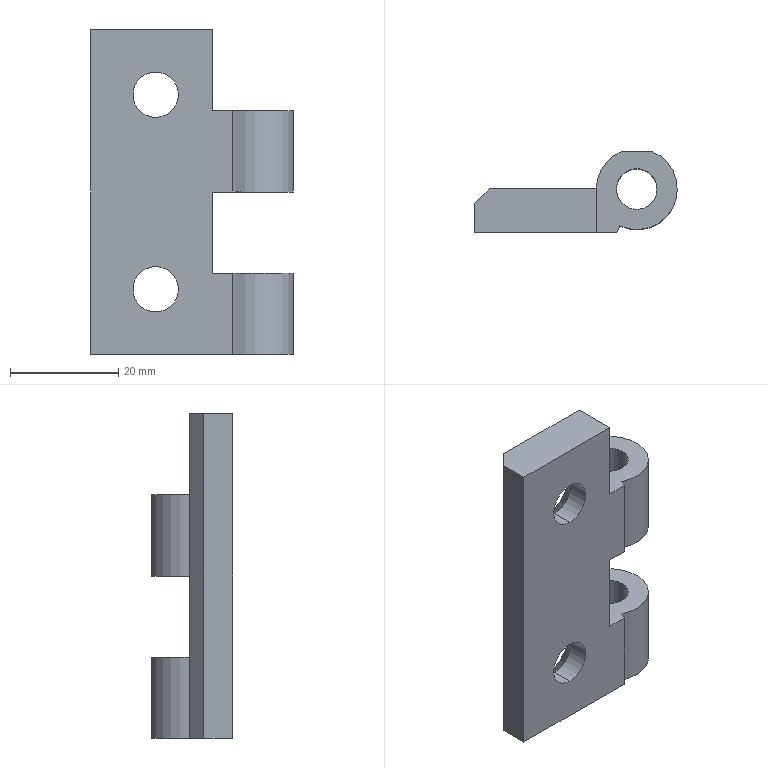Part | SolidWorks | features BaseBody 1 | 1 solid | 31 faces | box 37.5 x 15 x 60 mm | volume 13445 mm3 | plane 15 | cylinder 12 | cone 4 | commonest cylinder face diameters 7.5 x4 8.4 x4 15 x4
STEP:
#1=CARTESIAN_POINT('',(-18.,-4.05,-7.8));
#2=VERTEX_POINT('',#1);
#3=CARTESIAN_POINT('',(-18.,-4.05,-16.2));
#4=VERTEX_POINT('',#3);
#5=CARTESIAN_POINT('',(-18.,-4.05,-12.));
#6=DIRECTION('',(0.,-1.,0.));
#7=DIRECTION('',(0.,0.,-1.));
#8=AXIS2_PLACEMENT_3D('',#5,#6,#7);
#9=CIRCLE('',#8,4.2);
#10=EDGE_CURVE('',#2,#4,#9,.T.);
#11=ORIENTED_EDGE('',*,*,#10,.F.);
#12=CARTESIAN_POINT('',(-18.,-8.,-7.8));
#13=VERTEX_POINT('',#12);
#14=CARTESIAN_POINT('',(-18.,50.,-7.8));
#15=DIRECTION('',(0.,-1.,0.));
#16=VECTOR('',#15,1000.);
#17=LINE('',#14,#16);
#18=EDGE_CURVE('',#2,#13,#17,.T.);
#19=ORIENTED_EDGE('',*,*,#18,.T.);
#20=CARTESIAN_POINT('',(-18.,-8.,-16.2));
#21=VERTEX_POINT('',#20);
#22=CARTESIAN_POINT('',(-18.,-8.,-12.));
#23=DIRECTION('',(0.,-1.,0.));
#24=DIRECTION('',(0.,0.,-1.));
#25=AXIS2_PLACEMENT_3D('',#22,#23,#24);
#26=CIRCLE('',#25,4.2);
#27=EDGE_CURVE('',#13,#21,#26,.T.);
#28=ORIENTED_EDGE('',*,*,#27,.T.);
#29=CARTESIAN_POINT('',(-18.,50.,-16.2));
#30=DIRECTION('',(0.,-1.,0.));
#31=VECTOR('',#30,1000.);
#32=LINE('',#29,#31);
#33=EDGE_CURVE('',#4,#21,#32,.T.);
#34=ORIENTED_EDGE('',*,*,#33,.F.);
#35=EDGE_LOOP('',(#11,#19,#28,#34));
#36=FACE_OUTER_BOUND('',#35,.T.);
#37=CARTESIAN_POINT('',(-18.,50.,-12.));
#38=DIRECTION('',(0.,-1.,0.));
#39=DIRECTION('',(0.,0.,-1.));
#40=AXIS2_PLACEMENT_3D('',#37,#38,#39);
#41=CYLINDRICAL_SURFACE('',#40,4.2);
#42=ADVANCED_FACE('',(#36),#41,.F.);
#43=CARTESIAN_POINT('',(-18.,-4.05,-43.8));
#44=VERTEX_POINT('',#43);
#45=CARTESIAN_POINT('',(-18.,-4.05,-52.2));
#46=VERTEX_POINT('',#45);
#47=CARTESIAN_POINT('',(-18.,-4.05,-48.));
#48=DIRECTION('',(0.,-1.,0.));
#49=DIRECTION('',(0.,0.,-1.));
#50=AXIS2_PLACEMENT_3D('',#47,#48,#49);
#51=CIRCLE('',#50,4.2);
#52=EDGE_CURVE('',#44,#46,#51,.T.);
#53=ORIENTED_EDGE('',*,*,#52,.F.);
#54=CARTESIAN_POINT('',(-18.,-8.,-43.8));
#55=VERTEX_POINT('',#54);
#56=CARTESIAN_POINT('',(-18.,50.,-43.8));
#57=DIRECTION('',(0.,-1.,0.));
#58=VECTOR('',#57,1000.);
#59=LINE('',#56,#58);
#60=EDGE_CURVE('',#44,#55,#59,.T.);
#61=ORIENTED_EDGE('',*,*,#60,.T.);
#62=CARTESIAN_POINT('',(-18.,-8.,-52.2));
#63=VERTEX_POINT('',#62);
#64=CARTESIAN_POINT('',(-18.,-8.,-48.));
#65=DIRECTION('',(0.,-1.,0.));
#66=DIRECTION('',(0.,0.,-1.));
#67=AXIS2_PLACEMENT_3D('',#64,#65,#66);
#68=CIRCLE('',#67,4.2);
#69=EDGE_CURVE('',#55,#63,#68,.T.);
#70=ORIENTED_EDGE('',*,*,#69,.T.);
#71=CARTESIAN_POINT('',(-18.,50.,-52.2));
#72=DIRECTION('',(0.,-1.,0.));
#73=VECTOR('',#72,1000.);
#74=LINE('',#71,#73);
#75=EDGE_CURVE('',#46,#63,#74,.T.);
#76=ORIENTED_EDGE('',*,*,#75,.F.);
#77=EDGE_LOOP('',(#53,#61,#70,#76));
#78=FACE_OUTER_BOUND('',#77,.T.);
#79=CARTESIAN_POINT('',(-18.,50.,-48.));
#80=DIRECTION('',(0.,-1.,0.));
#81=DIRECTION('',(0.,0.,-1.));
#82=AXIS2_PLACEMENT_3D('',#79,#80,#81);
#83=CYLINDRICAL_SURFACE('',#82,4.2);
#84=ADVANCED_FACE('',(#78),#83,.F.);
#85=ORIENTED_EDGE('',*,*,#10,.T.);
#86=CARTESIAN_POINT('',(-18.,0.,-20.25));
#87=VERTEX_POINT('',#86);
#88=CARTESIAN_POINT('',(-18.,0.,-20.25));
#89=DIRECTION('',(0.,0.7071,-0.7071));
#90=VECTOR('',#89,1000.);
#91=LINE('',#88,#90);
#92=EDGE_CURVE('',#4,#87,#91,.T.);
#93=ORIENTED_EDGE('',*,*,#92,.T.);
#94=CARTESIAN_POINT('',(-18.,0.,-3.75));
#95=VERTEX_POINT('',#94);
#96=CARTESIAN_POINT('',(-18.,0.,-12.));
#97=DIRECTION('',(0.,-1.,0.));
#98=DIRECTION('',(0.,0.,1.));
#99=AXIS2_PLACEMENT_3D('',#96,#97,#98);
#100=CIRCLE('',#99,8.25);
#101=EDGE_CURVE('',#95,#87,#100,.T.);
#102=ORIENTED_EDGE('',*,*,#101,.F.);
#103=CARTESIAN_POINT('',(-18.,0.,-3.75));
#104=DIRECTION('',(0.,0.7071,0.7071));
#105=VECTOR('',#104,1000.);
#106=LINE('',#103,#105);
#107=EDGE_CURVE('',#2,#95,#106,.T.);
#108=ORIENTED_EDGE('',*,*,#107,.F.);
#109=EDGE_LOOP('',(#85,#93,#102,#108));
#110=FACE_OUTER_BOUND('',#109,.T.);
#111=CARTESIAN_POINT('',(-18.,0.,-12.));
#112=DIRECTION('',(0.,1.,0.));
#113=DIRECTION('',(0.,0.,1.));
#114=AXIS2_PLACEMENT_3D('',#111,#112,#113);
#115=CONICAL_SURFACE('',#114,8.25,0.7854);
#116=ADVANCED_FACE('',(#110),#115,.F.);
#117=ORIENTED_EDGE('',*,*,#52,.T.);
#118=CARTESIAN_POINT('',(-18.,0.,-56.25));
#119=VERTEX_POINT('',#118);
#120=CARTESIAN_POINT('',(-18.,0.,-56.25));
#121=DIRECTION('',(0.,0.7071,-0.7071));
#122=VECTOR('',#121,1000.);
#123=LINE('',#120,#122);
#124=EDGE_CURVE('',#46,#119,#123,.T.);
#125=ORIENTED_EDGE('',*,*,#124,.T.);
#126=CARTESIAN_POINT('',(-18.,0.,-39.75));
#127=VERTEX_POINT('',#126);
#128=CARTESIAN_POINT('',(-18.,0.,-48.));
#129=DIRECTION('',(0.,-1.,0.));
#130=DIRECTION('',(0.,0.,1.));
#131=AXIS2_PLACEMENT_3D('',#128,#129,#130);
#132=CIRCLE('',#131,8.25);
#133=EDGE_CURVE('',#127,#119,#132,.T.);
#134=ORIENTED_EDGE('',*,*,#133,.F.);
#135=CARTESIAN_POINT('',(-18.,0.,-39.75));
#136=DIRECTION('',(0.,0.7071,0.7071));
#137=VECTOR('',#136,1000.);
#138=LINE('',#135,#137);
#139=EDGE_CURVE('',#44,#127,#138,.T.);
#140=ORIENTED_EDGE('',*,*,#139,.F.);
#141=EDGE_LOOP('',(#117,#125,#134,#140));
#142=FACE_OUTER_BOUND('',#141,.T.);
#143=CARTESIAN_POINT('',(-18.,0.,-48.));
#144=DIRECTION('',(0.,1.,0.));
#145=DIRECTION('',(0.,0.,1.));
#146=AXIS2_PLACEMENT_3D('',#143,#144,#145);
#147=CONICAL_SURFACE('',#146,8.25,0.7854);
#148=ADVANCED_FACE('',(#142),#147,.F.);
#149=CARTESIAN_POINT('',(3.75,0.,-45.));
#150=VERTEX_POINT('',#149);
#151=CARTESIAN_POINT('',(-3.75,0.,-45.));
#152=VERTEX_POINT('',#151);
#153=CARTESIAN_POINT('',(0.,0.,-45.));
#154=DIRECTION('',(0.,0.,-1.));
#155=DIRECTION('',(-1.,0.,0.));
#156=AXIS2_PLACEMENT_3D('',#153,#154,#155);
#157=CIRCLE('',#156,3.75);
#158=EDGE_CURVE('',#150,#152,#157,.T.);
#159=ORIENTED_EDGE('',*,*,#158,.F.);
#160=CARTESIAN_POINT('',(3.75,0.,-60.));
#161=VERTEX_POINT('',#160);
#162=CARTESIAN_POINT('',(3.75,0.,-60.));
#163=DIRECTION('',(0.,0.,-1.));
#164=VECTOR('',#163,1000.);
#165=LINE('',#162,#164);
#166=EDGE_CURVE('',#150,#161,#165,.T.);
#167=ORIENTED_EDGE('',*,*,#166,.T.);
#168=CARTESIAN_POINT('',(-3.75,0.,-60.));
#169=VERTEX_POINT('',#168);
#170=CARTESIAN_POINT('',(0.,0.,-60.));
#171=DIRECTION('',(0.,0.,1.));
#172=DIRECTION('',(-1.,0.,0.));
#173=AXIS2_PLACEMENT_3D('',#170,#171,#172);
#174=CIRCLE('',#173,3.75);
#175=EDGE_CURVE('',#169,#161,#174,.T.);
#176=ORIENTED_EDGE('',*,*,#175,.F.);
#177=CARTESIAN_POINT('',(-3.75,0.,-60.));
#178=DIRECTION('',(0.,0.,-1.));
#179=VECTOR('',#178,1000.);
#180=LINE('',#177,#179);
#181=EDGE_CURVE('',#152,#169,#180,.T.);
#182=ORIENTED_EDGE('',*,*,#181,.F.);
#183=EDGE_LOOP('',(#159,#167,#176,#182));
#184=FACE_OUTER_BOUND('',#183,.T.);
#185=CARTESIAN_POINT('',(0.,0.,-60.));
#186=DIRECTION('',(0.,0.,-1.));
#187=DIRECTION('',(-1.,0.,0.));
#188=AXIS2_PLACEMENT_3D('',#185,#186,#187);
#189=CYLINDRICAL_SURFACE('',#188,3.75);
#190=ADVANCED_FACE('',(#184),#189,.F.);
#191=CARTESIAN_POINT('',(3.75,0.,-15.));
#192=VERTEX_POINT('',#191);
#193=CARTESIAN_POINT('',(-3.75,0.,-15.));
#194=VERTEX_POINT('',#193);
#195=CARTESIAN_POINT('',(0.,0.,-15.));
#196=DIRECTION('',(0.,0.,-1.));
#197=DIRECTION('',(-1.,0.,0.));
#198=AXIS2_PLACEMENT_3D('',#195,#196,#197);
#199=CIRCLE('',#198,3.75);
#200=EDGE_CURVE('',#192,#194,#199,.T.);
#201=ORIENTED_EDGE('',*,*,#200,.F.);
#202=CARTESIAN_POINT('',(3.75,0.,-30.));
#203=VERTEX_POINT('',#202);
#204=CARTESIAN_POINT('',(3.75,0.,-60.));
#205=DIRECTION('',(0.,0.,-1.));
#206=VECTOR('',#205,1000.);
#207=LINE('',#204,#206);
#208=EDGE_CURVE('',#192,#203,#207,.T.);
#209=ORIENTED_EDGE('',*,*,#208,.T.);
#210=CARTESIAN_POINT('',(-3.75,0.,-30.));
#211=VERTEX_POINT('',#210);
#212=CARTESIAN_POINT('',(0.,0.,-30.));
#213=DIRECTION('',(0.,0.,1.));
#214=DIRECTION('',(-1.,0.,0.));
#215=AXIS2_PLACEMENT_3D('',#212,#213,#214);
#216=CIRCLE('',#215,3.75);
#217=EDGE_CURVE('',#211,#203,#216,.T.);
#218=ORIENTED_EDGE('',*,*,#217,.F.);
#219=CARTESIAN_POINT('',(-3.75,0.,-60.));
#220=DIRECTION('',(0.,0.,-1.));
#221=VECTOR('',#220,1000.);
#222=LINE('',#219,#221);
#223=EDGE_CURVE('',#194,#211,#222,.T.);
#224=ORIENTED_EDGE('',*,*,#223,.F.);
#225=EDGE_LOOP('',(#201,#209,#218,#224));
#226=FACE_OUTER_BOUND('',#225,.T.);
#227=CARTESIAN_POINT('',(0.,0.,-60.));
#228=DIRECTION('',(0.,0.,-1.));
#229=DIRECTION('',(-1.,0.,0.));
#230=AXIS2_PLACEMENT_3D('',#227,#228,#229);
#231=CYLINDRICAL_SURFACE('',#230,3.75);
#232=ADVANCED_FACE('',(#226),#231,.F.);
#233=CARTESIAN_POINT('',(-18.,-8.,-12.));
#234=DIRECTION('',(0.,-1.,0.));
#235=DIRECTION('',(0.,0.,-1.));
#236=AXIS2_PLACEMENT_3D('',#233,#234,#235);
#237=CIRCLE('',#236,4.2);
#238=EDGE_CURVE('',#21,#13,#237,.T.);
#239=ORIENTED_EDGE('',*,*,#238,.F.);
#240=ORIENTED_EDGE('',*,*,#27,.F.);
#241=EDGE_LOOP('',(#239,#240));
#242=FACE_BOUND('',#241,.T.);
#243=CARTESIAN_POINT('',(-18.,-8.,-48.));
#244=DIRECTION('',(0.,-1.,0.));
#245=DIRECTION('',(0.,0.,-1.));
#246=AXIS2_PLACEMENT_3D('',#243,#244,#245);
#247=CIRCLE('',#246,4.2);
#248=EDGE_CURVE('',#63,#55,#247,.T.);
#249=ORIENTED_EDGE('',*,*,#248,.F.);
#250=ORIENTED_EDGE('',*,*,#69,.F.);
#251=EDGE_LOOP('',(#249,#250));
#252=FACE_BOUND('',#251,.T.);
#253=CARTESIAN_POINT('',(-7.5,-8.,-30.));
#254=VERTEX_POINT('',#253);
#255=CARTESIAN_POINT('',(-7.5,-8.,-45.));
#256=VERTEX_POINT('',#255);
#257=CARTESIAN_POINT('',(-7.5,-8.,-60.));
#258=DIRECTION('',(0.,0.,-1.));
#259=VECTOR('',#258,1000.);
#260=LINE('',#257,#259);
#261=EDGE_CURVE('',#254,#256,#260,.T.);
#262=ORIENTED_EDGE('',*,*,#261,.F.);
#263=CARTESIAN_POINT('',(-3.75,-8.,-30.));
#264=VERTEX_POINT('',#263);
#265=CARTESIAN_POINT('',(-3.75,-8.,-30.));
#266=DIRECTION('',(-1.,0.,0.));
#267=VECTOR('',#266,1000.);
#268=LINE('',#265,#267);
#269=EDGE_CURVE('',#264,#254,#268,.T.);
#270=ORIENTED_EDGE('',*,*,#269,.F.);
#271=CARTESIAN_POINT('',(-3.75,-8.,-15.));
#272=VERTEX_POINT('',#271);
#273=CARTESIAN_POINT('',(-3.75,-8.,-60.));
#274=DIRECTION('',(0.,0.,-1.));
#275=VECTOR('',#274,1000.);
#276=LINE('',#273,#275);
#277=EDGE_CURVE('',#272,#264,#276,.T.);
#278=ORIENTED_EDGE('',*,*,#277,.F.);
#279=CARTESIAN_POINT('',(-7.5,-8.,-15.));
#280=VERTEX_POINT('',#279);
#281=CARTESIAN_POINT('',(-3.75,-8.,-15.));
#282=DIRECTION('',(1.,0.,0.));
#283=VECTOR('',#282,1000.);
#284=LINE('',#281,#283);
#285=EDGE_CURVE('',#280,#272,#284,.T.);
#286=ORIENTED_EDGE('',*,*,#285,.F.);
#287=CARTESIAN_POINT('',(-7.5,-8.,0.));
#288=VERTEX_POINT('',#287);
#289=CARTESIAN_POINT('',(-7.5,-8.,-60.));
#290=DIRECTION('',(0.,0.,-1.));
#291=VECTOR('',#290,1000.);
#292=LINE('',#289,#291);
#293=EDGE_CURVE('',#288,#280,#292,.T.);
#294=ORIENTED_EDGE('',*,*,#293,.F.);
#295=CARTESIAN_POINT('',(-30.,-8.,0.));
#296=VERTEX_POINT('',#295);
#297=CARTESIAN_POINT('',(-3.75,-8.,0.));
#298=DIRECTION('',(1.,0.,0.));
#299=VECTOR('',#298,1000.);
#300=LINE('',#297,#299);
#301=EDGE_CURVE('',#296,#288,#300,.T.);
#302=ORIENTED_EDGE('',*,*,#301,.F.);
#303=CARTESIAN_POINT('',(-30.,-8.,-60.));
#304=VERTEX_POINT('',#303);
#305=CARTESIAN_POINT('',(-30.,-8.,-60.));
#306=DIRECTION('',(0.,0.,1.));
#307=VECTOR('',#306,1000.);
#308=LINE('',#305,#307);
#309=EDGE_CURVE('',#304,#296,#308,.T.);
#310=ORIENTED_EDGE('',*,*,#309,.F.);
#311=CARTESIAN_POINT('',(-3.75,-8.,-60.));
#312=VERTEX_POINT('',#311);
#313=CARTESIAN_POINT('',(-3.75,-8.,-60.));
#314=DIRECTION('',(-1.,0.,0.));
#315=VECTOR('',#314,1000.);
#316=LINE('',#313,#315);
#317=EDGE_CURVE('',#312,#304,#316,.T.);
#318=ORIENTED_EDGE('',*,*,#317,.F.);
#319=CARTESIAN_POINT('',(-3.75,-8.,-45.));
#320=VERTEX_POINT('',#319);
#321=CARTESIAN_POINT('',(-3.75,-8.,-60.));
#322=DIRECTION('',(0.,0.,-1.));
#323=VECTOR('',#322,1000.);
#324=LINE('',#321,#323);
#325=EDGE_CURVE('',#320,#312,#324,.T.);
#326=ORIENTED_EDGE('',*,*,#325,.F.);
#327=CARTESIAN_POINT('',(-3.75,-8.,-45.));
#328=DIRECTION('',(1.,0.,0.));
#329=VECTOR('',#328,1000.);
#330=LINE('',#327,#329);
#331=EDGE_CURVE('',#256,#320,#330,.T.);
#332=ORIENTED_EDGE('',*,*,#331,.F.);
#333=EDGE_LOOP('',(#262,#270,#278,#286,#294,#302,#310,#318,#326,#332));
#334=FACE_OUTER_BOUND('',#333,.T.);
#335=CARTESIAN_POINT('',(-3.75,-8.,-60.));
#336=DIRECTION('',(0.,1.,0.));
#337=DIRECTION('',(0.,0.,1.));
#338=AXIS2_PLACEMENT_3D('',#335,#336,#337);
#339=PLANE('',#338);
#340=ADVANCED_FACE('',(#242,#252,#334),#339,.F.);
#341=ORIENTED_EDGE('',*,*,#18,.F.);
#342=CARTESIAN_POINT('',(-18.,-4.05,-12.));
#343=DIRECTION('',(0.,-1.,0.));
#344=DIRECTION('',(0.,0.,-1.));
#345=AXIS2_PLACEMENT_3D('',#342,#343,#344);
#346=CIRCLE('',#345,4.2);
#347=EDGE_CURVE('',#4,#2,#346,.T.);
#348=ORIENTED_EDGE('',*,*,#347,.F.);
#349=ORIENTED_EDGE('',*,*,#33,.T.);
#350=ORIENTED_EDGE('',*,*,#238,.T.);
#351=EDGE_LOOP('',(#341,#348,#349,#350));
#352=FACE_OUTER_BOUND('',#351,.T.);
#353=CARTESIAN_POINT('',(-18.,50.,-12.));
#354=DIRECTION('',(0.,-1.,0.));
#355=DIRECTION('',(0.,0.,-1.));
#356=AXIS2_PLACEMENT_3D('',#353,#354,#355);
#357=CYLINDRICAL_SURFACE('',#356,4.2);
#358=ADVANCED_FACE('',(#352),#357,.F.);
#359=ORIENTED_EDGE('',*,*,#60,.F.);
#360=CARTESIAN_POINT('',(-18.,-4.05,-48.));
#361=DIRECTION('',(0.,-1.,0.));
#362=DIRECTION('',(0.,0.,-1.));
#363=AXIS2_PLACEMENT_3D('',#360,#361,#362);
#364=CIRCLE('',#363,4.2);
#365=EDGE_CURVE('',#46,#44,#364,.T.);
#366=ORIENTED_EDGE('',*,*,#365,.F.);
#367=ORIENTED_EDGE('',*,*,#75,.T.);
#368=ORIENTED_EDGE('',*,*,#248,.T.);
#369=EDGE_LOOP('',(#359,#366,#367,#368));
#370=FACE_OUTER_BOUND('',#369,.T.);
#371=CARTESIAN_POINT('',(-18.,50.,-48.));
#372=DIRECTION('',(0.,-1.,0.));
#373=DIRECTION('',(0.,0.,-1.));
#374=AXIS2_PLACEMENT_3D('',#371,#372,#373);
#375=CYLINDRICAL_SURFACE('',#374,4.2);
#376=ADVANCED_FACE('',(#370),#375,.F.);
#377=CARTESIAN_POINT('',(0.,0.,-45.));
#378=DIRECTION('',(0.,0.,-1.));
#379=DIRECTION('',(-1.,0.,0.));
#380=AXIS2_PLACEMENT_3D('',#377,#378,#379);
#381=CIRCLE('',#380,3.75);
#382=EDGE_CURVE('',#152,#150,#381,.T.);
#383=ORIENTED_EDGE('',*,*,#382,.T.);
#384=ORIENTED_EDGE('',*,*,#158,.T.);
#385=EDGE_LOOP('',(#383,#384));
#386=FACE_BOUND('',#385,.T.);
#387=CARTESIAN_POINT('',(-2.693,7.,-45.));
#388=VERTEX_POINT('',#387);
#389=CARTESIAN_POINT('',(-7.5,0.,-45.));
#390=VERTEX_POINT('',#389);
#391=CARTESIAN_POINT('',(0.,0.,-45.));
#392=DIRECTION('',(0.,0.,1.));
#393=DIRECTION('',(-1.,0.,0.));
#394=AXIS2_PLACEMENT_3D('',#391,#392,#393);
#395=CIRCLE('',#394,7.5);
#396=EDGE_CURVE('',#388,#390,#395,.T.);
#397=ORIENTED_EDGE('',*,*,#396,.T.);
#398=CARTESIAN_POINT('',(-7.5,15.,-45.));
#399=DIRECTION('',(0.,-1.,0.));
#400=VECTOR('',#399,1000.);
#401=LINE('',#398,#400);
#402=EDGE_CURVE('',#390,#256,#401,.T.);
#403=ORIENTED_EDGE('',*,*,#402,.T.);
#404=ORIENTED_EDGE('',*,*,#331,.T.);
#405=CARTESIAN_POINT('',(-3.148,-6.808,-45.));
#406=VERTEX_POINT('',#405);
#407=CARTESIAN_POINT('',(-3.75,-8.,-45.));
#408=DIRECTION('',(0.451,0.8925,0.));
#409=VECTOR('',#408,1000.);
#410=LINE('',#407,#409);
#411=EDGE_CURVE('',#320,#406,#410,.T.);
#412=ORIENTED_EDGE('',*,*,#411,.T.);
#413=CARTESIAN_POINT('',(2.693,7.,-45.));
#414=VERTEX_POINT('',#413);
#415=CARTESIAN_POINT('',(0.,0.,-45.));
#416=DIRECTION('',(0.,0.,1.));
#417=DIRECTION('',(-1.,0.,0.));
#418=AXIS2_PLACEMENT_3D('',#415,#416,#417);
#419=CIRCLE('',#418,7.5);
#420=EDGE_CURVE('',#406,#414,#419,.T.);
#421=ORIENTED_EDGE('',*,*,#420,.T.);
#422=CARTESIAN_POINT('',(7.5,7.,-45.));
#423=DIRECTION('',(-1.,0.,0.));
#424=VECTOR('',#423,1000.);
#425=LINE('',#422,#424);
#426=EDGE_CURVE('',#414,#388,#425,.T.);
#427=ORIENTED_EDGE('',*,*,#426,.T.);
#428=EDGE_LOOP('',(#397,#403,#404,#412,#421,#427));
#429=FACE_OUTER_BOUND('',#428,.T.);
#430=CARTESIAN_POINT('',(7.5,15.,-45.));
#431=DIRECTION('',(0.,0.,1.));
#432=DIRECTION('',(1.,0.,0.));
#433=AXIS2_PLACEMENT_3D('',#430,#431,#432);
#434=PLANE('',#433);
#435=ADVANCED_FACE('',(#386,#429),#434,.T.);
#436=CARTESIAN_POINT('',(-7.5,0.,-30.));
#437=VERTEX_POINT('',#436);
#438=CARTESIAN_POINT('',(-7.5,0.,-45.));
#439=DIRECTION('',(0.,0.,1.));
#440=VECTOR('',#439,1000.);
#441=LINE('',#438,#440);
#442=EDGE_CURVE('',#390,#437,#441,.T.);
#443=ORIENTED_EDGE('',*,*,#442,.T.);
#444=CARTESIAN_POINT('',(-7.5,15.,-30.));
#445=DIRECTION('',(0.,-1.,0.));
#446=VECTOR('',#445,1000.);
#447=LINE('',#444,#446);
#448=EDGE_CURVE('',#437,#254,#447,.T.);
#449=ORIENTED_EDGE('',*,*,#448,.T.);
#450=ORIENTED_EDGE('',*,*,#261,.T.);
#451=ORIENTED_EDGE('',*,*,#402,.F.);
#452=EDGE_LOOP('',(#443,#449,#450,#451));
#453=FACE_OUTER_BOUND('',#452,.T.);
#454=CARTESIAN_POINT('',(-7.5,15.,-45.));
#455=DIRECTION('',(1.,0.,0.));
#456=DIRECTION('',(0.,0.,-1.));
#457=AXIS2_PLACEMENT_3D('',#454,#455,#456);
#458=PLANE('',#457);
#459=ADVANCED_FACE('',(#453),#458,.T.);
#460=ORIENTED_EDGE('',*,*,#217,.T.);
#461=CARTESIAN_POINT('',(0.,0.,-30.));
#462=DIRECTION('',(0.,0.,1.));
#463=DIRECTION('',(-1.,0.,0.));
#464=AXIS2_PLACEMENT_3D('',#461,#462,#463);
#465=CIRCLE('',#464,3.75);
#466=EDGE_CURVE('',#203,#211,#465,.T.);
#467=ORIENTED_EDGE('',*,*,#466,.T.);
#468=EDGE_LOOP('',(#460,#467));
#469=FACE_BOUND('',#468,.T.);
#470=CARTESIAN_POINT('',(2.693,7.,-30.));
#471=VERTEX_POINT('',#470);
#472=CARTESIAN_POINT('',(-3.148,-6.808,-30.));
#473=VERTEX_POINT('',#472);
#474=CARTESIAN_POINT('',(0.,0.,-30.));
#475=DIRECTION('',(0.,0.,-1.));
#476=DIRECTION('',(-1.,0.,0.));
#477=AXIS2_PLACEMENT_3D('',#474,#475,#476);
#478=CIRCLE('',#477,7.5);
#479=EDGE_CURVE('',#471,#473,#478,.T.);
#480=ORIENTED_EDGE('',*,*,#479,.T.);
#481=CARTESIAN_POINT('',(-3.148,-6.808,-30.));
#482=DIRECTION('',(-0.451,-0.8925,0.));
#483=VECTOR('',#482,1000.);
#484=LINE('',#481,#483);
#485=EDGE_CURVE('',#473,#264,#484,.T.);
#486=ORIENTED_EDGE('',*,*,#485,.T.);
#487=ORIENTED_EDGE('',*,*,#269,.T.);
#488=ORIENTED_EDGE('',*,*,#448,.F.);
#489=CARTESIAN_POINT('',(-2.693,7.,-30.));
#490=VERTEX_POINT('',#489);
#491=CARTESIAN_POINT('',(0.,0.,-30.));
#492=DIRECTION('',(0.,0.,-1.));
#493=DIRECTION('',(-1.,0.,0.));
#494=AXIS2_PLACEMENT_3D('',#491,#492,#493);
#495=CIRCLE('',#494,7.5);
#496=EDGE_CURVE('',#437,#490,#495,.T.);
#497=ORIENTED_EDGE('',*,*,#496,.T.);
#498=CARTESIAN_POINT('',(-7.5,7.,-30.));
#499=DIRECTION('',(1.,0.,0.));
#500=VECTOR('',#499,1000.);
#501=LINE('',#498,#500);
#502=EDGE_CURVE('',#490,#471,#501,.T.);
#503=ORIENTED_EDGE('',*,*,#502,.T.);
#504=EDGE_LOOP('',(#480,#486,#487,#488,#497,#503));
#505=FACE_OUTER_BOUND('',#504,.T.);
#506=CARTESIAN_POINT('',(-7.5,15.,-30.));
#507=DIRECTION('',(0.,0.,-1.));
#508=DIRECTION('',(-1.,0.,0.));
#509=AXIS2_PLACEMENT_3D('',#506,#507,#508);
#510=PLANE('',#509);
#511=ADVANCED_FACE('',(#469,#505),#510,.T.);
#512=CARTESIAN_POINT('',(-3.148,-6.808,-15.));
#513=VERTEX_POINT('',#512);
#514=CARTESIAN_POINT('',(-3.148,-6.808,-60.));
#515=DIRECTION('',(0.,0.,-1.));
#516=VECTOR('',#515,1000.);
#517=LINE('',#514,#516);
#518=EDGE_CURVE('',#513,#473,#517,.T.);
#519=ORIENTED_EDGE('',*,*,#518,.F.);
#520=CARTESIAN_POINT('',(-3.148,-6.808,-15.));
#521=DIRECTION('',(0.451,0.8925,0.));
#522=VECTOR('',#521,1000.);
#523=LINE('',#520,#522);
#524=EDGE_CURVE('',#272,#513,#523,.T.);
#525=ORIENTED_EDGE('',*,*,#524,.F.);
#526=ORIENTED_EDGE('',*,*,#277,.T.);
#527=ORIENTED_EDGE('',*,*,#485,.F.);
#528=EDGE_LOOP('',(#519,#525,#526,#527));
#529=FACE_OUTER_BOUND('',#528,.T.);
#530=CARTESIAN_POINT('',(-3.148,-6.808,-60.));
#531=DIRECTION('',(-0.8925,0.451,0.));
#532=DIRECTION('',(-0.451,-0.8925,0.));
#533=AXIS2_PLACEMENT_3D('',#530,#531,#532);
#534=PLANE('',#533);
#535=ADVANCED_FACE('',(#529),#534,.F.);
#536=CARTESIAN_POINT('',(0.,0.,-15.));
#537=DIRECTION('',(0.,0.,-1.));
#538=DIRECTION('',(-1.,0.,0.));
#539=AXIS2_PLACEMENT_3D('',#536,#537,#538);
#540=CIRCLE('',#539,3.75);
#541=EDGE_CURVE('',#194,#192,#540,.T.);
#542=ORIENTED_EDGE('',*,*,#541,.T.);
#543=ORIENTED_EDGE('',*,*,#200,.T.);
#544=EDGE_LOOP('',(#542,#543));
#545=FACE_BOUND('',#544,.T.);
#546=CARTESIAN_POINT('',(-2.693,7.,-15.));
#547=VERTEX_POINT('',#546);
#548=CARTESIAN_POINT('',(-7.5,0.,-15.));
#549=VERTEX_POINT('',#548);
#550=CARTESIAN_POINT('',(0.,0.,-15.));
#551=DIRECTION('',(0.,0.,1.));
#552=DIRECTION('',(-1.,0.,0.));
#553=AXIS2_PLACEMENT_3D('',#550,#551,#552);
#554=CIRCLE('',#553,7.5);
#555=EDGE_CURVE('',#547,#549,#554,.T.);
#556=ORIENTED_EDGE('',*,*,#555,.T.);
#557=CARTESIAN_POINT('',(-7.5,15.,-15.));
#558=DIRECTION('',(0.,-1.,0.));
#559=VECTOR('',#558,1000.);
#560=LINE('',#557,#559);
#561=EDGE_CURVE('',#549,#280,#560,.T.);
#562=ORIENTED_EDGE('',*,*,#561,.T.);
#563=ORIENTED_EDGE('',*,*,#285,.T.);
#564=ORIENTED_EDGE('',*,*,#524,.T.);
#565=CARTESIAN_POINT('',(2.693,7.,-15.));
#566=VERTEX_POINT('',#565);
#567=CARTESIAN_POINT('',(0.,0.,-15.));
#568=DIRECTION('',(0.,0.,1.));
#569=DIRECTION('',(-1.,0.,0.));
#570=AXIS2_PLACEMENT_3D('',#567,#568,#569);
#571=CIRCLE('',#570,7.5);
#572=EDGE_CURVE('',#513,#566,#571,.T.);
#573=ORIENTED_EDGE('',*,*,#572,.T.);
#574=CARTESIAN_POINT('',(7.5,7.,-15.));
#575=DIRECTION('',(-1.,0.,0.));
#576=VECTOR('',#575,1000.);
#577=LINE('',#574,#576);
#578=EDGE_CURVE('',#566,#547,#577,.T.);
#579=ORIENTED_EDGE('',*,*,#578,.T.);
#580=EDGE_LOOP('',(#556,#562,#563,#564,#573,#579));
#581=FACE_OUTER_BOUND('',#580,.T.);
#582=CARTESIAN_POINT('',(7.5,15.,-15.));
#583=DIRECTION('',(0.,0.,1.));
#584=DIRECTION('',(1.,0.,0.));
#585=AXIS2_PLACEMENT_3D('',#582,#583,#584);
#586=PLANE('',#585);
#587=ADVANCED_FACE('',(#545,#581),#586,.T.);
#588=CARTESIAN_POINT('',(-7.5,0.,0.));
#589=VERTEX_POINT('',#588);
#590=CARTESIAN_POINT('',(-7.5,0.,-15.));
#591=DIRECTION('',(0.,0.,1.));
#592=VECTOR('',#591,1000.);
#593=LINE('',#590,#592);
#594=EDGE_CURVE('',#549,#589,#593,.T.);
#595=ORIENTED_EDGE('',*,*,#594,.T.);
#596=CARTESIAN_POINT('',(-7.5,15.,0.));
#597=DIRECTION('',(0.,-1.,0.));
#598=VECTOR('',#597,1000.);
#599=LINE('',#596,#598);
#600=EDGE_CURVE('',#589,#288,#599,.T.);
#601=ORIENTED_EDGE('',*,*,#600,.T.);
#602=ORIENTED_EDGE('',*,*,#293,.T.);
#603=ORIENTED_EDGE('',*,*,#561,.F.);
#604=EDGE_LOOP('',(#595,#601,#602,#603));
#605=FACE_OUTER_BOUND('',#604,.T.);
#606=CARTESIAN_POINT('',(-7.5,15.,-15.));
#607=DIRECTION('',(1.,0.,0.));
#608=DIRECTION('',(0.,0.,-1.));
#609=AXIS2_PLACEMENT_3D('',#606,#607,#608);
#610=PLANE('',#609);
#611=ADVANCED_FACE('',(#605),#610,.T.);
#612=CARTESIAN_POINT('',(-27.333,0.,0.));
#613=VERTEX_POINT('',#612);
#614=CARTESIAN_POINT('',(0.,0.,0.));
#615=DIRECTION('',(1.,0.,0.));
#616=VECTOR('',#615,1000.);
#617=LINE('',#614,#616);
#618=EDGE_CURVE('',#613,#589,#617,.T.);
#619=ORIENTED_EDGE('',*,*,#618,.F.);
#620=CARTESIAN_POINT('',(-30.,-2.667,0.));
#621=VERTEX_POINT('',#620);
#622=CARTESIAN_POINT('',(-30.,-2.667,0.));
#623=DIRECTION('',(0.7071,0.7071,0.));
#624=VECTOR('',#623,1000.);
#625=LINE('',#622,#624);
#626=EDGE_CURVE('',#621,#613,#625,.T.);
#627=ORIENTED_EDGE('',*,*,#626,.F.);
#628=CARTESIAN_POINT('',(-30.,0.,0.));
#629=DIRECTION('',(0.,1.,0.));
#630=VECTOR('',#629,1000.);
#631=LINE('',#628,#630);
#632=EDGE_CURVE('',#296,#621,#631,.T.);
#633=ORIENTED_EDGE('',*,*,#632,.F.);
#634=ORIENTED_EDGE('',*,*,#301,.T.);
#635=ORIENTED_EDGE('',*,*,#600,.F.);
#636=EDGE_LOOP('',(#619,#627,#633,#634,#635));
#637=FACE_OUTER_BOUND('',#636,.T.);
#638=CARTESIAN_POINT('',(0.,0.,0.));
#639=DIRECTION('',(0.,0.,-1.));
#640=DIRECTION('',(-1.,0.,0.));
#641=AXIS2_PLACEMENT_3D('',#638,#639,#640);
#642=PLANE('',#641);
#643=ADVANCED_FACE('',(#637),#642,.F.);
#644=CARTESIAN_POINT('',(-30.,-2.667,-60.));
#645=VERTEX_POINT('',#644);
#646=CARTESIAN_POINT('',(-30.,-2.667,-60.));
#647=DIRECTION('',(0.,0.,1.));
#648=VECTOR('',#647,1000.);
#649=LINE('',#646,#648);
#650=EDGE_CURVE('',#645,#621,#649,.T.);
#651=ORIENTED_EDGE('',*,*,#650,.F.);
#652=CARTESIAN_POINT('',(-30.,-8.,-60.));
#653=DIRECTION('',(0.,1.,0.));
#654=VECTOR('',#653,1000.);
#655=LINE('',#652,#654);
#656=EDGE_CURVE('',#304,#645,#655,.T.);
#657=ORIENTED_EDGE('',*,*,#656,.F.);
#658=ORIENTED_EDGE('',*,*,#309,.T.);
#659=ORIENTED_EDGE('',*,*,#632,.T.);
#660=EDGE_LOOP('',(#651,#657,#658,#659));
#661=FACE_OUTER_BOUND('',#660,.T.);
#662=CARTESIAN_POINT('',(-30.,-8.,-60.));
#663=DIRECTION('',(1.,0.,0.));
#664=DIRECTION('',(0.,1.,0.));
#665=AXIS2_PLACEMENT_3D('',#662,#663,#664);
#666=PLANE('',#665);
#667=ADVANCED_FACE('',(#661),#666,.F.);
#668=ORIENTED_EDGE('',*,*,#175,.T.);
#669=CARTESIAN_POINT('',(0.,0.,-60.));
#670=DIRECTION('',(0.,0.,1.));
#671=DIRECTION('',(-1.,0.,0.));
#672=AXIS2_PLACEMENT_3D('',#669,#670,#671);
#673=CIRCLE('',#672,3.75);
#674=EDGE_CURVE('',#161,#169,#673,.T.);
#675=ORIENTED_EDGE('',*,*,#674,.T.);
#676=EDGE_LOOP('',(#668,#675));
#677=FACE_BOUND('',#676,.T.);
#678=CARTESIAN_POINT('',(-27.333,0.,-60.));
#679=VERTEX_POINT('',#678);
#680=CARTESIAN_POINT('',(-7.5,0.,-60.));
#681=VERTEX_POINT('',#680);
#682=CARTESIAN_POINT('',(0.,0.,-60.));
#683=DIRECTION('',(1.,0.,0.));
#684=VECTOR('',#683,1000.);
#685=LINE('',#682,#684);
#686=EDGE_CURVE('',#679,#681,#685,.T.);
#687=ORIENTED_EDGE('',*,*,#686,.T.);
#688=CARTESIAN_POINT('',(-2.693,7.,-60.));
#689=VERTEX_POINT('',#688);
#690=CARTESIAN_POINT('',(0.,0.,-60.));
#691=DIRECTION('',(0.,0.,-1.));
#692=DIRECTION('',(-1.,0.,0.));
#693=AXIS2_PLACEMENT_3D('',#690,#691,#692);
#694=CIRCLE('',#693,7.5);
#695=EDGE_CURVE('',#681,#689,#694,.T.);
#696=ORIENTED_EDGE('',*,*,#695,.T.);
#697=CARTESIAN_POINT('',(2.693,7.,-60.));
#698=VERTEX_POINT('',#697);
#699=CARTESIAN_POINT('',(0.,7.,-60.));
#700=DIRECTION('',(1.,0.,0.));
#701=VECTOR('',#700,1000.);
#702=LINE('',#699,#701);
#703=EDGE_CURVE('',#689,#698,#702,.T.);
#704=ORIENTED_EDGE('',*,*,#703,.T.);
#705=CARTESIAN_POINT('',(-3.148,-6.808,-60.));
#706=VERTEX_POINT('',#705);
#707=CARTESIAN_POINT('',(0.,0.,-60.));
#708=DIRECTION('',(0.,0.,-1.));
#709=DIRECTION('',(-1.,0.,0.));
#710=AXIS2_PLACEMENT_3D('',#707,#708,#709);
#711=CIRCLE('',#710,7.5);
#712=EDGE_CURVE('',#698,#706,#711,.T.);
#713=ORIENTED_EDGE('',*,*,#712,.T.);
#714=CARTESIAN_POINT('',(-3.148,-6.808,-60.));
#715=DIRECTION('',(-0.451,-0.8925,0.));
#716=VECTOR('',#715,1000.);
#717=LINE('',#714,#716);
#718=EDGE_CURVE('',#706,#312,#717,.T.);
#719=ORIENTED_EDGE('',*,*,#718,.T.);
#720=ORIENTED_EDGE('',*,*,#317,.T.);
#721=ORIENTED_EDGE('',*,*,#656,.T.);
#722=CARTESIAN_POINT('',(-30.,-2.667,-60.));
#723=DIRECTION('',(0.7071,0.7071,0.));
#724=VECTOR('',#723,1000.);
#725=LINE('',#722,#724);
#726=EDGE_CURVE('',#645,#679,#725,.T.);
#727=ORIENTED_EDGE('',*,*,#726,.T.);
#728=EDGE_LOOP('',(#687,#696,#704,#713,#719,#720,#721,#727));
#729=FACE_OUTER_BOUND('',#728,.T.);
#730=CARTESIAN_POINT('',(0.,0.,-60.));
#731=DIRECTION('',(0.,0.,-1.));
#732=DIRECTION('',(-1.,0.,0.));
#733=AXIS2_PLACEMENT_3D('',#730,#731,#732);
#734=PLANE('',#733);
#735=ADVANCED_FACE('',(#677,#729),#734,.T.);
#736=ORIENTED_EDGE('',*,*,#325,.T.);
#737=ORIENTED_EDGE('',*,*,#718,.F.);
#738=CARTESIAN_POINT('',(-3.148,-6.808,-60.));
#739=DIRECTION('',(0.,0.,-1.));
#740=VECTOR('',#739,1000.);
#741=LINE('',#738,#740);
#742=EDGE_CURVE('',#406,#706,#741,.T.);
#743=ORIENTED_EDGE('',*,*,#742,.F.);
#744=ORIENTED_EDGE('',*,*,#411,.F.);
#745=EDGE_LOOP('',(#736,#737,#743,#744));
#746=FACE_OUTER_BOUND('',#745,.T.);
#747=CARTESIAN_POINT('',(-3.148,-6.808,-60.));
#748=DIRECTION('',(-0.8925,0.451,0.));
#749=DIRECTION('',(-0.451,-0.8925,0.));
#750=AXIS2_PLACEMENT_3D('',#747,#748,#749);
#751=PLANE('',#750);
#752=ADVANCED_FACE('',(#746),#751,.F.);
#753=ORIENTED_EDGE('',*,*,#92,.F.);
#754=ORIENTED_EDGE('',*,*,#347,.T.);
#755=ORIENTED_EDGE('',*,*,#107,.T.);
#756=CARTESIAN_POINT('',(-18.,0.,-12.));
#757=DIRECTION('',(0.,-1.,0.));
#758=DIRECTION('',(0.,0.,1.));
#759=AXIS2_PLACEMENT_3D('',#756,#757,#758);
#760=CIRCLE('',#759,8.25);
#761=EDGE_CURVE('',#87,#95,#760,.T.);
#762=ORIENTED_EDGE('',*,*,#761,.F.);
#763=EDGE_LOOP('',(#753,#754,#755,#762));
#764=FACE_OUTER_BOUND('',#763,.T.);
#765=CARTESIAN_POINT('',(-18.,0.,-12.));
#766=DIRECTION('',(0.,1.,0.));
#767=DIRECTION('',(0.,0.,1.));
#768=AXIS2_PLACEMENT_3D('',#765,#766,#767);
#769=CONICAL_SURFACE('',#768,8.25,0.7854);
#770=ADVANCED_FACE('',(#764),#769,.F.);
#771=ORIENTED_EDGE('',*,*,#124,.F.);
#772=ORIENTED_EDGE('',*,*,#365,.T.);
#773=ORIENTED_EDGE('',*,*,#139,.T.);
#774=CARTESIAN_POINT('',(-18.,0.,-48.));
#775=DIRECTION('',(0.,-1.,0.));
#776=DIRECTION('',(0.,0.,1.));
#777=AXIS2_PLACEMENT_3D('',#774,#775,#776);
#778=CIRCLE('',#777,8.25);
#779=EDGE_CURVE('',#119,#127,#778,.T.);
#780=ORIENTED_EDGE('',*,*,#779,.F.);
#781=EDGE_LOOP('',(#771,#772,#773,#780));
#782=FACE_OUTER_BOUND('',#781,.T.);
#783=CARTESIAN_POINT('',(-18.,0.,-48.));
#784=DIRECTION('',(0.,1.,0.));
#785=DIRECTION('',(0.,0.,1.));
#786=AXIS2_PLACEMENT_3D('',#783,#784,#785);
#787=CONICAL_SURFACE('',#786,8.25,0.7854);
#788=ADVANCED_FACE('',(#782),#787,.F.);
#789=ORIENTED_EDGE('',*,*,#166,.F.);
#790=ORIENTED_EDGE('',*,*,#382,.F.);
#791=ORIENTED_EDGE('',*,*,#181,.T.);
#792=ORIENTED_EDGE('',*,*,#674,.F.);
#793=EDGE_LOOP('',(#789,#790,#791,#792));
#794=FACE_OUTER_BOUND('',#793,.T.);
#795=CARTESIAN_POINT('',(0.,0.,-60.));
#796=DIRECTION('',(0.,0.,-1.));
#797=DIRECTION('',(-1.,0.,0.));
#798=AXIS2_PLACEMENT_3D('',#795,#796,#797);
#799=CYLINDRICAL_SURFACE('',#798,3.75);
#800=ADVANCED_FACE('',(#794),#799,.F.);
#801=ORIENTED_EDGE('',*,*,#695,.F.);
#802=CARTESIAN_POINT('',(-7.5,0.,-60.));
#803=DIRECTION('',(0.,0.,1.));
#804=VECTOR('',#803,1000.);
#805=LINE('',#802,#804);
#806=EDGE_CURVE('',#681,#390,#805,.T.);
#807=ORIENTED_EDGE('',*,*,#806,.T.);
#808=ORIENTED_EDGE('',*,*,#396,.F.);
#809=CARTESIAN_POINT('',(-2.693,7.,-60.));
#810=DIRECTION('',(0.,0.,-1.));
#811=VECTOR('',#810,1000.);
#812=LINE('',#809,#811);
#813=EDGE_CURVE('',#388,#689,#812,.T.);
#814=ORIENTED_EDGE('',*,*,#813,.T.);
#815=EDGE_LOOP('',(#801,#807,#808,#814));
#816=FACE_OUTER_BOUND('',#815,.T.);
#817=CARTESIAN_POINT('',(0.,0.,-60.));
#818=DIRECTION('',(0.,0.,-1.));
#819=DIRECTION('',(-1.,0.,0.));
#820=AXIS2_PLACEMENT_3D('',#817,#818,#819);
#821=CYLINDRICAL_SURFACE('',#820,7.5);
#822=ADVANCED_FACE('',(#816),#821,.T.);
#823=CARTESIAN_POINT('',(2.693,7.,-60.));
#824=DIRECTION('',(0.,0.,1.));
#825=VECTOR('',#824,1000.);
#826=LINE('',#823,#825);
#827=EDGE_CURVE('',#698,#414,#826,.T.);
#828=ORIENTED_EDGE('',*,*,#827,.F.);
#829=ORIENTED_EDGE('',*,*,#703,.F.);
#830=ORIENTED_EDGE('',*,*,#813,.F.);
#831=ORIENTED_EDGE('',*,*,#426,.F.);
#832=EDGE_LOOP('',(#828,#829,#830,#831));
#833=FACE_OUTER_BOUND('',#832,.T.);
#834=CARTESIAN_POINT('',(-2.693,7.,-60.));
#835=DIRECTION('',(0.,-1.,0.));
#836=DIRECTION('',(0.,0.,-1.));
#837=AXIS2_PLACEMENT_3D('',#834,#835,#836);
#838=PLANE('',#837);
#839=ADVANCED_FACE('',(#833),#838,.F.);
#840=ORIENTED_EDGE('',*,*,#712,.F.);
#841=ORIENTED_EDGE('',*,*,#827,.T.);
#842=ORIENTED_EDGE('',*,*,#420,.F.);
#843=ORIENTED_EDGE('',*,*,#742,.T.);
#844=EDGE_LOOP('',(#840,#841,#842,#843));
#845=FACE_OUTER_BOUND('',#844,.T.);
#846=CARTESIAN_POINT('',(0.,0.,-60.));
#847=DIRECTION('',(0.,0.,-1.));
#848=DIRECTION('',(-1.,0.,0.));
#849=AXIS2_PLACEMENT_3D('',#846,#847,#848);
#850=CYLINDRICAL_SURFACE('',#849,7.5);
#851=ADVANCED_FACE('',(#845),#850,.T.);
#852=ORIENTED_EDGE('',*,*,#101,.T.);
#853=ORIENTED_EDGE('',*,*,#761,.T.);
#854=EDGE_LOOP('',(#852,#853));
#855=FACE_BOUND('',#854,.T.);
#856=ORIENTED_EDGE('',*,*,#133,.T.);
#857=ORIENTED_EDGE('',*,*,#779,.T.);
#858=EDGE_LOOP('',(#856,#857));
#859=FACE_BOUND('',#858,.T.);
#860=ORIENTED_EDGE('',*,*,#594,.F.);
#861=CARTESIAN_POINT('',(-7.5,0.,-60.));
#862=DIRECTION('',(0.,0.,1.));
#863=VECTOR('',#862,1000.);
#864=LINE('',#861,#863);
#865=EDGE_CURVE('',#437,#549,#864,.T.);
#866=ORIENTED_EDGE('',*,*,#865,.F.);
#867=ORIENTED_EDGE('',*,*,#442,.F.);
#868=ORIENTED_EDGE('',*,*,#806,.F.);
#869=ORIENTED_EDGE('',*,*,#686,.F.);
#870=CARTESIAN_POINT('',(-27.333,0.,-60.));
#871=DIRECTION('',(0.,0.,-1.));
#872=VECTOR('',#871,1000.);
#873=LINE('',#870,#872);
#874=EDGE_CURVE('',#613,#679,#873,.T.);
#875=ORIENTED_EDGE('',*,*,#874,.F.);
#876=ORIENTED_EDGE('',*,*,#618,.T.);
#877=EDGE_LOOP('',(#860,#866,#867,#868,#869,#875,#876));
#878=FACE_OUTER_BOUND('',#877,.T.);
#879=CARTESIAN_POINT('',(-27.333,0.,-60.));
#880=DIRECTION('',(0.,-1.,0.));
#881=DIRECTION('',(0.,0.,-1.));
#882=AXIS2_PLACEMENT_3D('',#879,#880,#881);
#883=PLANE('',#882);
#884=ADVANCED_FACE('',(#855,#859,#878),#883,.F.);
#885=ORIENTED_EDGE('',*,*,#208,.F.);
#886=ORIENTED_EDGE('',*,*,#541,.F.);
#887=ORIENTED_EDGE('',*,*,#223,.T.);
#888=ORIENTED_EDGE('',*,*,#466,.F.);
#889=EDGE_LOOP('',(#885,#886,#887,#888));
#890=FACE_OUTER_BOUND('',#889,.T.);
#891=CARTESIAN_POINT('',(0.,0.,-60.));
#892=DIRECTION('',(0.,0.,-1.));
#893=DIRECTION('',(-1.,0.,0.));
#894=AXIS2_PLACEMENT_3D('',#891,#892,#893);
#895=CYLINDRICAL_SURFACE('',#894,3.75);
#896=ADVANCED_FACE('',(#890),#895,.F.);
#897=ORIENTED_EDGE('',*,*,#518,.T.);
#898=ORIENTED_EDGE('',*,*,#479,.F.);
#899=CARTESIAN_POINT('',(2.693,7.,-60.));
#900=DIRECTION('',(0.,0.,1.));
#901=VECTOR('',#900,1000.);
#902=LINE('',#899,#901);
#903=EDGE_CURVE('',#471,#566,#902,.T.);
#904=ORIENTED_EDGE('',*,*,#903,.T.);
#905=ORIENTED_EDGE('',*,*,#572,.F.);
#906=EDGE_LOOP('',(#897,#898,#904,#905));
#907=FACE_OUTER_BOUND('',#906,.T.);
#908=CARTESIAN_POINT('',(0.,0.,-60.));
#909=DIRECTION('',(0.,0.,-1.));
#910=DIRECTION('',(-1.,0.,0.));
#911=AXIS2_PLACEMENT_3D('',#908,#909,#910);
#912=CYLINDRICAL_SURFACE('',#911,7.5);
#913=ADVANCED_FACE('',(#907),#912,.T.);
#914=CARTESIAN_POINT('',(-2.693,7.,-60.));
#915=DIRECTION('',(0.,0.,-1.));
#916=VECTOR('',#915,1000.);
#917=LINE('',#914,#916);
#918=EDGE_CURVE('',#547,#490,#917,.T.);
#919=ORIENTED_EDGE('',*,*,#918,.F.);
#920=ORIENTED_EDGE('',*,*,#578,.F.);
#921=ORIENTED_EDGE('',*,*,#903,.F.);
#922=ORIENTED_EDGE('',*,*,#502,.F.);
#923=EDGE_LOOP('',(#919,#920,#921,#922));
#924=FACE_OUTER_BOUND('',#923,.T.);
#925=CARTESIAN_POINT('',(-2.693,7.,-60.));
#926=DIRECTION('',(0.,-1.,0.));
#927=DIRECTION('',(0.,0.,-1.));
#928=AXIS2_PLACEMENT_3D('',#925,#926,#927);
#929=PLANE('',#928);
#930=ADVANCED_FACE('',(#924),#929,.F.);
#931=ORIENTED_EDGE('',*,*,#555,.F.);
#932=ORIENTED_EDGE('',*,*,#918,.T.);
#933=ORIENTED_EDGE('',*,*,#496,.F.);
#934=ORIENTED_EDGE('',*,*,#865,.T.);
#935=EDGE_LOOP('',(#931,#932,#933,#934));
#936=FACE_OUTER_BOUND('',#935,.T.);
#937=CARTESIAN_POINT('',(0.,0.,-60.));
#938=DIRECTION('',(0.,0.,-1.));
#939=DIRECTION('',(-1.,0.,0.));
#940=AXIS2_PLACEMENT_3D('',#937,#938,#939);
#941=CYLINDRICAL_SURFACE('',#940,7.5);
#942=ADVANCED_FACE('',(#936),#941,.T.);
#943=ORIENTED_EDGE('',*,*,#874,.T.);
#944=ORIENTED_EDGE('',*,*,#726,.F.);
#945=ORIENTED_EDGE('',*,*,#650,.T.);
#946=ORIENTED_EDGE('',*,*,#626,.T.);
#947=EDGE_LOOP('',(#943,#944,#945,#946));
#948=FACE_OUTER_BOUND('',#947,.T.);
#949=CARTESIAN_POINT('',(-30.,-2.667,-60.));
#950=DIRECTION('',(0.7071,-0.7071,0.));
#951=DIRECTION('',(0.7071,0.7071,0.));
#952=AXIS2_PLACEMENT_3D('',#949,#950,#951);
#953=PLANE('',#952);
#954=ADVANCED_FACE('',(#948),#953,.F.);
#955=CLOSED_SHELL('',(#42,#84,#116,#148,#190,#232,#340,#358,#376,#435,#459,#511,#535,#587,#611,#643,#667,#735,#752,#770,#788,#800,#822,#839,#851,#884,#896,#913,#930,#942,#954));
#956=MANIFOLD_SOLID_BREP('',#955);
#957=CARTESIAN_POINT('',(0.,0.,0.));
#958=DIRECTION('',(0.,0.,1.));
#959=DIRECTION('',(1.,0.,0.));
#960=AXIS2_PLACEMENT_3D('',#957,#958,#959);
#961=(LENGTH_UNIT()NAMED_UNIT(*)SI_UNIT(.MILLI.,.METRE.));
#962=UNCERTAINTY_MEASURE_WITH_UNIT(LENGTH_MEASURE(0.00001),#961,'','');
#963=(NAMED_UNIT(*)PLANE_ANGLE_UNIT()SI_UNIT($,.RADIAN.));
#964=(NAMED_UNIT(*)SI_UNIT($,.STERADIAN.)SOLID_ANGLE_UNIT());
#965=(GEOMETRIC_REPRESENTATION_CONTEXT(3)GLOBAL_UNCERTAINTY_ASSIGNED_CONTEXT((#962))GLOBAL_UNIT_ASSIGNED_CONTEXT((#961,#963,#964))REPRESENTATION_CONTEXT('',''));
#966=ADVANCED_BREP_SHAPE_REPRESENTATION('',(#956,#960),#965);